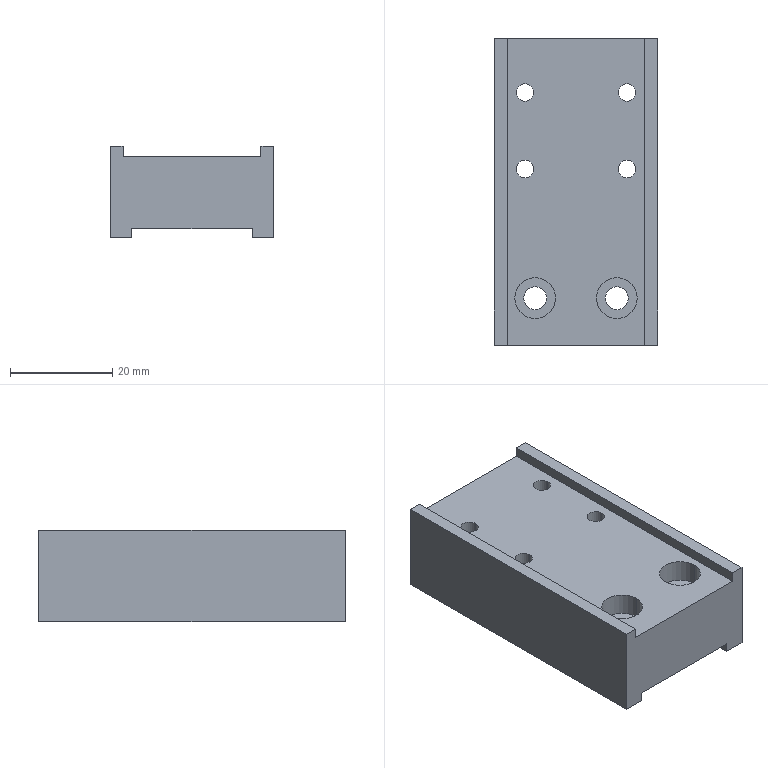Part | STEP file | A06 | 1 solid | 52 faces | box 32 x 60 x 18 mm | volume 26849 mm3 | cylinder 26 | plane 24 | cone 2 | commonest cylinder face diameters 3.4 x8 6.5 x8 4.5 x4 8 x4 5 x2